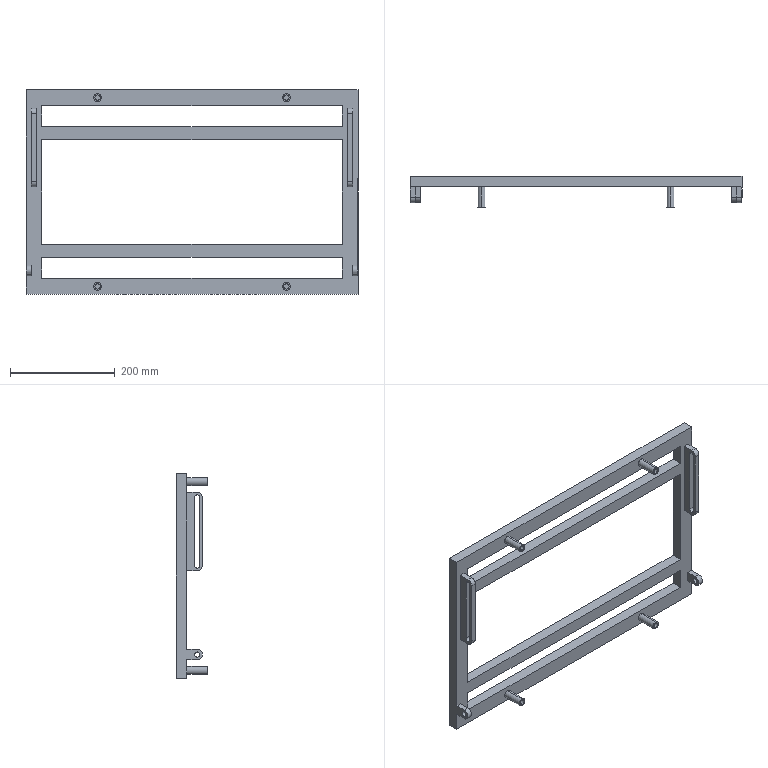Part | SolidWorks | 1 solid | 88 faces | box 634 x 60 x 390 mm | volume 1783210 mm3 | plane 56 | cylinder 32 | commonest cylinder face diameters 10 x18 15 x8 20 x6